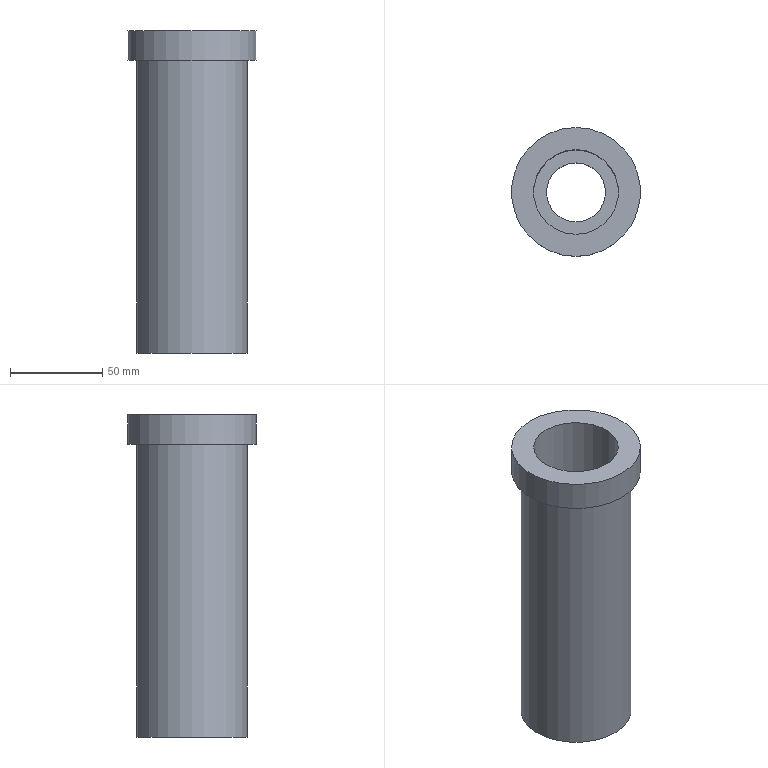Part | NX | features solid 2 | 1 solid | 8 faces | box 70 x 70 x 175 mm | volume 263187 mm3 | cylinder 4 | plane 4 | commonest cylinder face diameters 32 x1 46 x1 60 x1 70 x1
STEP:
#1=CARTESIAN_POINT('',(-515.,160.,-4.));
#2=VERTEX_POINT('',#1);
#3=CARTESIAN_POINT('',(-515.,190.,-4.));
#4=DIRECTION('',(0.,0.,-1.));
#5=DIRECTION('',(0.,-1.,0.));
#6=AXIS2_PLACEMENT_3D('',#3,#4,#5);
#7=CIRCLE('',#6,30.);
#8=EDGE_CURVE('',#2,#2,#7,.T.);
#9=ORIENTED_EDGE('',*,*,#8,.T.);
#10=EDGE_LOOP('',(#9));
#11=FACE_BOUND('',#10,.T.);
#12=CARTESIAN_POINT('',(-515.,160.,-163.));
#13=VERTEX_POINT('',#12);
#14=CARTESIAN_POINT('',(-515.,190.,-163.));
#15=DIRECTION('',(0.,0.,1.));
#16=DIRECTION('',(0.,-1.,0.));
#17=AXIS2_PLACEMENT_3D('',#14,#15,#16);
#18=CIRCLE('',#17,30.);
#19=EDGE_CURVE('',#13,#13,#18,.F.);
#20=ORIENTED_EDGE('',*,*,#19,.F.);
#21=EDGE_LOOP('',(#20));
#22=FACE_BOUND('',#21,.T.);
#23=CARTESIAN_POINT('',(-515.,190.,-68.));
#24=DIRECTION('',(0.,0.,1.));
#25=DIRECTION('',(0.,-1.,0.));
#26=AXIS2_PLACEMENT_3D('',#23,#24,#25);
#27=CYLINDRICAL_SURFACE('',#26,30.);
#28=ADVANCED_FACE('',(#11,#22),#27,.T.);
#29=CARTESIAN_POINT('',(-515.,167.,-113.));
#30=VERTEX_POINT('',#29);
#31=CARTESIAN_POINT('',(-515.,190.,-113.));
#32=DIRECTION('',(0.,0.,1.));
#33=DIRECTION('',(0.,-1.,0.));
#34=AXIS2_PLACEMENT_3D('',#31,#32,#33);
#35=CIRCLE('',#34,23.);
#36=EDGE_CURVE('',#30,#30,#35,.F.);
#37=ORIENTED_EDGE('',*,*,#36,.T.);
#38=EDGE_LOOP('',(#37));
#39=FACE_BOUND('',#38,.T.);
#40=CARTESIAN_POINT('',(-515.,167.,12.));
#41=VERTEX_POINT('',#40);
#42=CARTESIAN_POINT('',(-515.,190.,12.));
#43=DIRECTION('',(0.,0.,-1.));
#44=DIRECTION('',(0.,-1.,0.));
#45=AXIS2_PLACEMENT_3D('',#42,#43,#44);
#46=CIRCLE('',#45,23.);
#47=EDGE_CURVE('',#41,#41,#46,.T.);
#48=ORIENTED_EDGE('',*,*,#47,.F.);
#49=EDGE_LOOP('',(#48));
#50=FACE_BOUND('',#49,.T.);
#51=CARTESIAN_POINT('',(-515.,190.,-68.));
#52=DIRECTION('',(0.,0.,1.));
#53=DIRECTION('',(0.,-1.,0.));
#54=AXIS2_PLACEMENT_3D('',#51,#52,#53);
#55=CYLINDRICAL_SURFACE('',#54,23.);
#56=ADVANCED_FACE('',(#39,#50),#55,.F.);
#57=CARTESIAN_POINT('',(-515.,155.,12.));
#58=VERTEX_POINT('',#57);
#59=CARTESIAN_POINT('',(-515.,190.,12.));
#60=DIRECTION('',(0.,0.,-1.));
#61=DIRECTION('',(0.,-1.,0.));
#62=AXIS2_PLACEMENT_3D('',#59,#60,#61);
#63=CIRCLE('',#62,35.);
#64=EDGE_CURVE('',#58,#58,#63,.T.);
#65=ORIENTED_EDGE('',*,*,#64,.T.);
#66=EDGE_LOOP('',(#65));
#67=FACE_BOUND('',#66,.T.);
#68=CARTESIAN_POINT('',(-515.,155.,-4.));
#69=VERTEX_POINT('',#68);
#70=CARTESIAN_POINT('',(-515.,190.,-4.));
#71=DIRECTION('',(0.,0.,-1.));
#72=DIRECTION('',(0.,-1.,0.));
#73=AXIS2_PLACEMENT_3D('',#70,#71,#72);
#74=CIRCLE('',#73,35.);
#75=EDGE_CURVE('',#69,#69,#74,.T.);
#76=ORIENTED_EDGE('',*,*,#75,.F.);
#77=EDGE_LOOP('',(#76));
#78=FACE_BOUND('',#77,.T.);
#79=CARTESIAN_POINT('',(-515.,190.,8.));
#80=DIRECTION('',(0.,0.,-1.));
#81=DIRECTION('',(0.,1.,0.));
#82=AXIS2_PLACEMENT_3D('',#79,#80,#81);
#83=CYLINDRICAL_SURFACE('',#82,35.);
#84=ADVANCED_FACE('',(#67,#78),#83,.T.);
#85=ORIENTED_EDGE('',*,*,#64,.F.);
#86=EDGE_LOOP('',(#85));
#87=FACE_BOUND('',#86,.T.);
#88=ORIENTED_EDGE('',*,*,#47,.T.);
#89=EDGE_LOOP('',(#88));
#90=FACE_BOUND('',#89,.T.);
#91=CARTESIAN_POINT('',(-515.,190.,12.));
#92=DIRECTION('',(0.,0.,1.));
#93=DIRECTION('',(0.,-1.,0.));
#94=AXIS2_PLACEMENT_3D('',#91,#92,#93);
#95=PLANE('',#94);
#96=ADVANCED_FACE('',(#87,#90),#95,.T.);
#97=ORIENTED_EDGE('',*,*,#8,.F.);
#98=EDGE_LOOP('',(#97));
#99=FACE_BOUND('',#98,.T.);
#100=ORIENTED_EDGE('',*,*,#75,.T.);
#101=EDGE_LOOP('',(#100));
#102=FACE_BOUND('',#101,.T.);
#103=CARTESIAN_POINT('',(-515.,190.,-4.));
#104=DIRECTION('',(0.,0.,1.));
#105=DIRECTION('',(0.,-1.,0.));
#106=AXIS2_PLACEMENT_3D('',#103,#104,#105);
#107=PLANE('',#106);
#108=ADVANCED_FACE('',(#99,#102),#107,.F.);
#109=CARTESIAN_POINT('',(-515.,174.,-163.));
#110=VERTEX_POINT('',#109);
#111=CARTESIAN_POINT('',(-515.,190.,-163.));
#112=DIRECTION('',(0.,0.,1.));
#113=DIRECTION('',(0.,-1.,0.));
#114=AXIS2_PLACEMENT_3D('',#111,#112,#113);
#115=CIRCLE('',#114,16.);
#116=EDGE_CURVE('',#110,#110,#115,.F.);
#117=ORIENTED_EDGE('',*,*,#116,.T.);
#118=EDGE_LOOP('',(#117));
#119=FACE_BOUND('',#118,.T.);
#120=CARTESIAN_POINT('',(-515.,174.,-113.));
#121=VERTEX_POINT('',#120);
#122=CARTESIAN_POINT('',(-515.,190.,-113.));
#123=DIRECTION('',(0.,0.,1.));
#124=DIRECTION('',(0.,-1.,0.));
#125=AXIS2_PLACEMENT_3D('',#122,#123,#124);
#126=CIRCLE('',#125,16.);
#127=EDGE_CURVE('',#121,#121,#126,.F.);
#128=ORIENTED_EDGE('',*,*,#127,.F.);
#129=EDGE_LOOP('',(#128));
#130=FACE_BOUND('',#129,.T.);
#131=CARTESIAN_POINT('',(-515.,190.,-93.));
#132=DIRECTION('',(0.,0.,1.));
#133=DIRECTION('',(0.,-1.,0.));
#134=AXIS2_PLACEMENT_3D('',#131,#132,#133);
#135=CYLINDRICAL_SURFACE('',#134,16.);
#136=ADVANCED_FACE('',(#119,#130),#135,.F.);
#137=ORIENTED_EDGE('',*,*,#19,.T.);
#138=EDGE_LOOP('',(#137));
#139=FACE_BOUND('',#138,.T.);
#140=ORIENTED_EDGE('',*,*,#116,.F.);
#141=EDGE_LOOP('',(#140));
#142=FACE_BOUND('',#141,.T.);
#143=CARTESIAN_POINT('',(-515.,190.,-163.));
#144=DIRECTION('',(0.,0.,1.));
#145=DIRECTION('',(0.,-1.,0.));
#146=AXIS2_PLACEMENT_3D('',#143,#144,#145);
#147=PLANE('',#146);
#148=ADVANCED_FACE('',(#139,#142),#147,.F.);
#149=ORIENTED_EDGE('',*,*,#36,.F.);
#150=EDGE_LOOP('',(#149));
#151=FACE_BOUND('',#150,.T.);
#152=ORIENTED_EDGE('',*,*,#127,.T.);
#153=EDGE_LOOP('',(#152));
#154=FACE_BOUND('',#153,.T.);
#155=CARTESIAN_POINT('',(-515.,190.,-113.));
#156=DIRECTION('',(0.,0.,1.));
#157=DIRECTION('',(0.,-1.,0.));
#158=AXIS2_PLACEMENT_3D('',#155,#156,#157);
#159=PLANE('',#158);
#160=ADVANCED_FACE('',(#151,#154),#159,.T.);
#161=CLOSED_SHELL('',(#28,#56,#84,#96,#108,#136,#148,#160));
#162=MANIFOLD_SOLID_BREP('',#161);
#163=(LENGTH_UNIT()NAMED_UNIT(*)SI_UNIT(.MILLI.,.METRE.));
#164=UNCERTAINTY_MEASURE_WITH_UNIT(LENGTH_MEASURE(0.00001),#163,'','');
#165=(NAMED_UNIT(*)PLANE_ANGLE_UNIT()SI_UNIT($,.RADIAN.));
#166=(NAMED_UNIT(*)SI_UNIT($,.STERADIAN.)SOLID_ANGLE_UNIT());
#167=(GEOMETRIC_REPRESENTATION_CONTEXT(3)GLOBAL_UNCERTAINTY_ASSIGNED_CONTEXT((#164))GLOBAL_UNIT_ASSIGNED_CONTEXT((#163,#165,#166))REPRESENTATION_CONTEXT('',''));
#168=ADVANCED_BREP_SHAPE_REPRESENTATION('',(#162),#167);